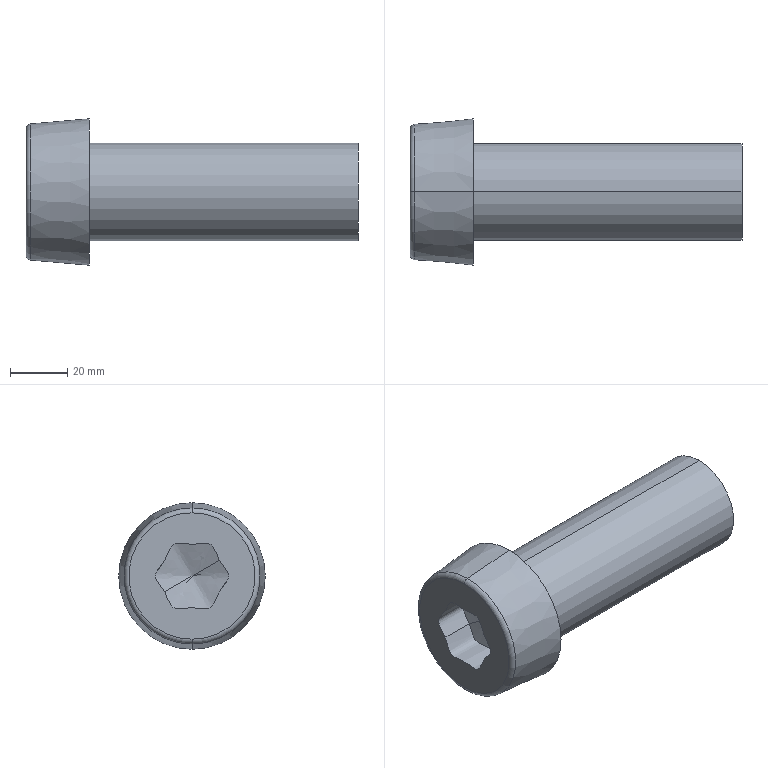Part | SolidWorks | features BlendCut 1, Cut 1, Extrusion 1, Fillet 1, LPattern 1, RevCut 1, Revolution 1, Scale 1 | 1 solid | 13 faces | box 115.6 x 51 x 51 mm | volume 120826 mm3 | spline 4 | plane 3 | torus 2 | cylinder 2 | cone 2 | commonest cylinder face diameters 34 x2
STEP:
#1=CARTESIAN_POINT('',(-21.403,-0.000002032,22.009));
#2=VERTEX_POINT('',#1);
#3=CARTESIAN_POINT('',(-21.403,-0.000002032,-22.009));
#4=VERTEX_POINT('',#3);
#5=CARTESIAN_POINT('',(-21.403,-0.000002032,0.000001814));
#6=DIRECTION('',(-1.,0.,0.));
#7=DIRECTION('',(0.,0.,-1.));
#8=AXIS2_PLACEMENT_3D('',#5,#6,#7);
#9=CIRCLE('',#8,22.009);
#10=EDGE_CURVE('',#2,#4,#9,.T.);
#11=ORIENTED_EDGE('',*,*,#10,.F.);
#12=CARTESIAN_POINT('',(-19.851,-0.000002032,23.702));
#13=VERTEX_POINT('',#12);
#14=CARTESIAN_POINT('',(-19.703,-0.000002032,22.009));
#15=DIRECTION('',(0.,1.,0.));
#16=DIRECTION('',(0.,0.,1.));
#17=AXIS2_PLACEMENT_3D('',#14,#15,#16);
#18=CIRCLE('',#17,1.7);
#19=EDGE_CURVE('',#2,#13,#18,.T.);
#20=ORIENTED_EDGE('',*,*,#19,.T.);
#21=CARTESIAN_POINT('',(-19.851,-0.000002032,-23.702));
#22=VERTEX_POINT('',#21);
#23=CARTESIAN_POINT('',(-19.851,-0.000002032,0.000001814));
#24=DIRECTION('',(1.,0.,0.));
#25=DIRECTION('',(0.,0.,-1.));
#26=AXIS2_PLACEMENT_3D('',#23,#24,#25);
#27=CIRCLE('',#26,23.702);
#28=EDGE_CURVE('',#22,#13,#27,.T.);
#29=ORIENTED_EDGE('',*,*,#28,.F.);
#30=CARTESIAN_POINT('',(-19.703,-0.000002032,-22.009));
#31=DIRECTION('',(0.,-1.,0.));
#32=DIRECTION('',(0.,0.,-1.));
#33=AXIS2_PLACEMENT_3D('',#30,#31,#32);
#34=CIRCLE('',#33,1.7);
#35=EDGE_CURVE('',#4,#22,#34,.T.);
#36=ORIENTED_EDGE('',*,*,#35,.F.);
#37=EDGE_LOOP('',(#11,#20,#29,#36));
#38=FACE_OUTER_BOUND('',#37,.T.);
#39=CARTESIAN_POINT('',(-19.703,-0.000002032,0.000001814));
#40=DIRECTION('',(1.,0.,0.));
#41=DIRECTION('',(0.,0.,-1.));
#42=AXIS2_PLACEMENT_3D('',#39,#40,#41);
#43=TOROIDAL_SURFACE('',#42,22.009,1.7);
#44=ADVANCED_FACE('',(#38),#43,.T.);
#45=CARTESIAN_POINT('',(-5.536,-0.000002032,0.000001814));
#46=VERTEX_POINT('',#45);
#47=CARTESIAN_POINT('',(-9.503,9.57,-5.525));
#48=VERTEX_POINT('',#47);
#49=CARTESIAN_POINT('',(-5.536,-0.000002032,0.000001814));
#50=CARTESIAN_POINT('',(-9.503,9.57,-5.525));
#51=B_SPLINE_CURVE_WITH_KNOTS('',1,(#49,#50),.UNSPECIFIED.,.F.,.F.,(2,2),(0.,1.),.UNSPECIFIED.);
#52=EDGE_CURVE('',#46,#48,#51,.T.);
#53=ORIENTED_EDGE('',*,*,#52,.F.);
#54=CARTESIAN_POINT('',(-9.503,-9.57,5.525));
#55=VERTEX_POINT('',#54);
#56=CARTESIAN_POINT('',(-5.536,-0.000002032,0.000001814));
#57=CARTESIAN_POINT('',(-9.503,-9.57,5.525));
#58=B_SPLINE_CURVE_WITH_KNOTS('',1,(#56,#57),.UNSPECIFIED.,.F.,.F.,(2,2),(0.,1.),.UNSPECIFIED.);
#59=EDGE_CURVE('',#46,#55,#58,.T.);
#60=ORIENTED_EDGE('',*,*,#59,.T.);
#61=CARTESIAN_POINT('',(-9.503,-9.57,5.525));
#62=CARTESIAN_POINT('',(-9.503,-8.343,7.65));
#63=CARTESIAN_POINT('',(-9.503,-7.361,12.75));
#64=CARTESIAN_POINT('',(-9.503,-0.000002032,10.2));
#65=CARTESIAN_POINT('',(-9.503,7.361,12.75));
#66=CARTESIAN_POINT('',(-9.503,8.833,5.1));
#67=CARTESIAN_POINT('',(-9.503,14.722,0.000001814));
#68=CARTESIAN_POINT('',(-9.503,10.796,-3.4));
#69=CARTESIAN_POINT('',(-9.503,9.57,-5.525));
#70=B_SPLINE_CURVE_WITH_KNOTS('',3,(#61,#62,#63,#64,#65,#66,#67,#68,#69),.UNSPECIFIED.,.F.,.F.,(4,1,1,1,1,1,4),(0.5,0.5833,0.6667,0.75,0.8333,0.9167,1.),.UNSPECIFIED.);
#71=EDGE_CURVE('',#55,#48,#70,.T.);
#72=ORIENTED_EDGE('',*,*,#71,.T.);
#73=EDGE_LOOP('',(#53,#60,#72));
#74=FACE_OUTER_BOUND('',#73,.T.);
#75=CARTESIAN_POINT('',(-5.536,-0.000002032,0.000001814));
#76=CARTESIAN_POINT('',(-9.503,9.57,-5.525));
#77=CARTESIAN_POINT('',(-5.536,-0.000002032,0.000001814));
#78=CARTESIAN_POINT('',(-9.503,8.343,-7.65));
#79=CARTESIAN_POINT('',(-5.536,-0.000002032,0.000001814));
#80=CARTESIAN_POINT('',(-9.503,7.361,-12.75));
#81=CARTESIAN_POINT('',(-5.536,-0.000002032,0.000001814));
#82=CARTESIAN_POINT('',(-9.503,-0.000002032,-10.2));
#83=CARTESIAN_POINT('',(-5.536,-0.000002032,0.000001814));
#84=CARTESIAN_POINT('',(-9.503,-7.361,-12.75));
#85=CARTESIAN_POINT('',(-5.536,-0.000002032,0.000001814));
#86=CARTESIAN_POINT('',(-9.503,-8.833,-5.1));
#87=CARTESIAN_POINT('',(-5.536,-0.000002032,0.000001814));
#88=CARTESIAN_POINT('',(-9.503,-14.722,0.000001814));
#89=CARTESIAN_POINT('',(-5.536,-0.000002032,0.000001814));
#90=CARTESIAN_POINT('',(-9.503,-8.833,5.1));
#91=CARTESIAN_POINT('',(-5.536,-0.000002032,0.000001814));
#92=CARTESIAN_POINT('',(-9.503,-7.361,12.75));
#93=CARTESIAN_POINT('',(-5.536,-0.000002032,0.000001814));
#94=CARTESIAN_POINT('',(-9.503,-0.000002032,10.2));
#95=CARTESIAN_POINT('',(-5.536,-0.000002032,0.000001814));
#96=CARTESIAN_POINT('',(-9.503,7.361,12.75));
#97=CARTESIAN_POINT('',(-5.536,-0.000002032,0.000001814));
#98=CARTESIAN_POINT('',(-9.503,8.833,5.1));
#99=CARTESIAN_POINT('',(-5.536,-0.000002032,0.000001814));
#100=CARTESIAN_POINT('',(-9.503,14.722,0.000001814));
#101=CARTESIAN_POINT('',(-5.536,-0.000002032,0.000001814));
#102=CARTESIAN_POINT('',(-9.503,10.796,-3.4));
#103=CARTESIAN_POINT('',(-5.536,-0.000002032,0.000001814));
#104=CARTESIAN_POINT('',(-9.503,9.57,-5.525));
#105=B_SPLINE_SURFACE_WITH_KNOTS('',3,1,((#75,#76),(#77,#78),(#79,#80),(#81,#82),(#83,#84),(#85,#86),(#87,#88),(#89,#90),(#91,#92),(#93,#94),(#95,#96),(#97,#98),(#99,#100),(#101,#102),(#103,#104)),.UNSPECIFIED.,.T.,.F.,.F.,(4,1,1,1,1,1,1,1,1,1,1,1,4),(2,2),(0.,0.08333,0.1667,0.25,0.3333,0.4167,0.5,0.5833,0.6667,0.75,0.8333,0.9167,1.),(0.,1.),.UNSPECIFIED.);
#106=ADVANCED_FACE('',(#74),#105,.F.);
#107=ORIENTED_EDGE('',*,*,#71,.F.);
#108=CARTESIAN_POINT('',(-21.403,-9.57,5.525));
#109=VERTEX_POINT('',#108);
#110=CARTESIAN_POINT('',(-9.503,-9.57,5.525));
#111=DIRECTION('',(-1.,0.,0.));
#112=VECTOR('',#111,1000.);
#113=LINE('',#110,#112);
#114=EDGE_CURVE('',#55,#109,#113,.T.);
#115=ORIENTED_EDGE('',*,*,#114,.T.);
#116=CARTESIAN_POINT('',(-21.403,9.57,-5.525));
#117=VERTEX_POINT('',#116);
#118=CARTESIAN_POINT('',(-21.403,9.57,-5.525));
#119=CARTESIAN_POINT('',(-21.403,10.796,-3.4));
#120=CARTESIAN_POINT('',(-21.403,14.722,0.000001814));
#121=CARTESIAN_POINT('',(-21.403,8.833,5.1));
#122=CARTESIAN_POINT('',(-21.403,7.361,12.75));
#123=CARTESIAN_POINT('',(-21.403,-0.000002032,10.2));
#124=CARTESIAN_POINT('',(-21.403,-7.361,12.75));
#125=CARTESIAN_POINT('',(-21.403,-8.343,7.65));
#126=CARTESIAN_POINT('',(-21.403,-9.57,5.525));
#127=B_SPLINE_CURVE_WITH_KNOTS('',3,(#118,#119,#120,#121,#122,#123,#124,#125,#126),.UNSPECIFIED.,.F.,.F.,(4,1,1,1,1,1,4),(0.,0.08333,0.1667,0.25,0.3333,0.4167,0.5),.UNSPECIFIED.);
#128=EDGE_CURVE('',#117,#109,#127,.T.);
#129=ORIENTED_EDGE('',*,*,#128,.F.);
#130=CARTESIAN_POINT('',(-9.503,9.57,-5.525));
#131=DIRECTION('',(-1.,0.,0.));
#132=VECTOR('',#131,1000.);
#133=LINE('',#130,#132);
#134=EDGE_CURVE('',#48,#117,#133,.T.);
#135=ORIENTED_EDGE('',*,*,#134,.F.);
#136=EDGE_LOOP('',(#107,#115,#129,#135));
#137=FACE_OUTER_BOUND('',#136,.T.);
#138=CARTESIAN_POINT('',(-9.503,9.57,-5.525));
#139=CARTESIAN_POINT('',(-21.403,9.57,-5.525));
#140=CARTESIAN_POINT('',(-9.503,10.796,-3.4));
#141=CARTESIAN_POINT('',(-21.403,10.796,-3.4));
#142=CARTESIAN_POINT('',(-9.503,14.722,0.000001814));
#143=CARTESIAN_POINT('',(-21.403,14.722,0.000001814));
#144=CARTESIAN_POINT('',(-9.503,8.833,5.1));
#145=CARTESIAN_POINT('',(-21.403,8.833,5.1));
#146=CARTESIAN_POINT('',(-9.503,7.361,12.75));
#147=CARTESIAN_POINT('',(-21.403,7.361,12.75));
#148=CARTESIAN_POINT('',(-9.503,-0.000002032,10.2));
#149=CARTESIAN_POINT('',(-21.403,-0.000002032,10.2));
#150=CARTESIAN_POINT('',(-9.503,-7.361,12.75));
#151=CARTESIAN_POINT('',(-21.403,-7.361,12.75));
#152=CARTESIAN_POINT('',(-9.503,-8.343,7.65));
#153=CARTESIAN_POINT('',(-21.403,-8.343,7.65));
#154=CARTESIAN_POINT('',(-9.503,-9.57,5.525));
#155=CARTESIAN_POINT('',(-21.403,-9.57,5.525));
#156=B_SPLINE_SURFACE_WITH_KNOTS('',3,1,((#138,#139),(#140,#141),(#142,#143),(#144,#145),(#146,#147),(#148,#149),(#150,#151),(#152,#153),(#154,#155)),.UNSPECIFIED.,.F.,.F.,.F.,(4,1,1,1,1,1,4),(2,2),(0.,0.08333,0.1667,0.25,0.3333,0.4167,0.5),(0.,1.),.UNSPECIFIED.);
#157=ADVANCED_FACE('',(#137),#156,.T.);
#158=CARTESIAN_POINT('',(94.197,-0.000002032,17.));
#159=VERTEX_POINT('',#158);
#160=CARTESIAN_POINT('',(94.197,-0.000002032,-17.));
#161=VERTEX_POINT('',#160);
#162=CARTESIAN_POINT('',(94.197,-0.000002032,0.000001814));
#163=DIRECTION('',(-1.,0.,0.));
#164=DIRECTION('',(0.,0.,1.));
#165=AXIS2_PLACEMENT_3D('',#162,#163,#164);
#166=CIRCLE('',#165,17.);
#167=EDGE_CURVE('',#159,#161,#166,.T.);
#168=ORIENTED_EDGE('',*,*,#167,.T.);
#169=CARTESIAN_POINT('',(0.6972,-0.000002032,-17.));
#170=VERTEX_POINT('',#169);
#171=CARTESIAN_POINT('',(-21.403,-0.000002032,-17.));
#172=DIRECTION('',(-1.,0.,0.));
#173=VECTOR('',#172,1000.);
#174=LINE('',#171,#173);
#175=EDGE_CURVE('',#161,#170,#174,.T.);
#176=ORIENTED_EDGE('',*,*,#175,.T.);
#177=CARTESIAN_POINT('',(0.6972,-0.000002032,17.));
#178=VERTEX_POINT('',#177);
#179=CARTESIAN_POINT('',(0.6972,-0.000002032,0.000001814));
#180=DIRECTION('',(-1.,0.,0.));
#181=DIRECTION('',(0.,0.,1.));
#182=AXIS2_PLACEMENT_3D('',#179,#180,#181);
#183=CIRCLE('',#182,17.);
#184=EDGE_CURVE('',#178,#170,#183,.T.);
#185=ORIENTED_EDGE('',*,*,#184,.F.);
#186=CARTESIAN_POINT('',(-21.403,-0.000002032,17.));
#187=DIRECTION('',(-1.,0.,0.));
#188=VECTOR('',#187,1000.);
#189=LINE('',#186,#188);
#190=EDGE_CURVE('',#159,#178,#189,.T.);
#191=ORIENTED_EDGE('',*,*,#190,.F.);
#192=EDGE_LOOP('',(#168,#176,#185,#191));
#193=FACE_OUTER_BOUND('',#192,.T.);
#194=CARTESIAN_POINT('',(-21.403,-0.000002032,0.000001814));
#195=DIRECTION('',(-1.,0.,0.));
#196=DIRECTION('',(0.,0.,1.));
#197=AXIS2_PLACEMENT_3D('',#194,#195,#196);
#198=CYLINDRICAL_SURFACE('',#197,17.);
#199=ADVANCED_FACE('',(#193),#198,.T.);
#200=ORIENTED_EDGE('',*,*,#28,.T.);
#201=CARTESIAN_POINT('',(0.6972,-0.000002032,25.5));
#202=VERTEX_POINT('',#201);
#203=CARTESIAN_POINT('',(0.6972,-0.000002032,25.5));
#204=DIRECTION('',(0.9962,0.,0.08716));
#205=VECTOR('',#204,1000.);
#206=LINE('',#203,#205);
#207=EDGE_CURVE('',#13,#202,#206,.T.);
#208=ORIENTED_EDGE('',*,*,#207,.T.);
#209=CARTESIAN_POINT('',(0.6972,-0.000002032,-25.5));
#210=VERTEX_POINT('',#209);
#211=CARTESIAN_POINT('',(0.6972,-0.000002032,0.000001814));
#212=DIRECTION('',(1.,0.,0.));
#213=DIRECTION('',(0.,0.,-1.));
#214=AXIS2_PLACEMENT_3D('',#211,#212,#213);
#215=CIRCLE('',#214,25.5);
#216=EDGE_CURVE('',#210,#202,#215,.T.);
#217=ORIENTED_EDGE('',*,*,#216,.F.);
#218=CARTESIAN_POINT('',(0.6972,-0.000002032,-25.5));
#219=DIRECTION('',(0.9962,0.,-0.08716));
#220=VECTOR('',#219,1000.);
#221=LINE('',#218,#220);
#222=EDGE_CURVE('',#22,#210,#221,.T.);
#223=ORIENTED_EDGE('',*,*,#222,.F.);
#224=EDGE_LOOP('',(#200,#208,#217,#223));
#225=FACE_OUTER_BOUND('',#224,.T.);
#226=CARTESIAN_POINT('',(0.6972,-0.000002032,0.000001814));
#227=DIRECTION('',(1.,0.,0.));
#228=DIRECTION('',(0.,0.,-1.));
#229=AXIS2_PLACEMENT_3D('',#226,#227,#228);
#230=CONICAL_SURFACE('',#229,25.5,0.08727);
#231=ADVANCED_FACE('',(#225),#230,.T.);
#232=CARTESIAN_POINT('',(-21.403,-0.000002032,0.000001814));
#233=DIRECTION('',(-1.,0.,0.));
#234=DIRECTION('',(0.,0.,-1.));
#235=AXIS2_PLACEMENT_3D('',#232,#233,#234);
#236=CIRCLE('',#235,22.009);
#237=EDGE_CURVE('',#4,#2,#236,.T.);
#238=ORIENTED_EDGE('',*,*,#237,.T.);
#239=ORIENTED_EDGE('',*,*,#10,.T.);
#240=EDGE_LOOP('',(#238,#239));
#241=FACE_OUTER_BOUND('',#240,.T.);
#242=ORIENTED_EDGE('',*,*,#128,.T.);
#243=CARTESIAN_POINT('',(-21.403,-9.57,5.525));
#244=CARTESIAN_POINT('',(-21.403,-10.796,3.4));
#245=CARTESIAN_POINT('',(-21.403,-14.722,0.000001814));
#246=CARTESIAN_POINT('',(-21.403,-8.833,-5.1));
#247=CARTESIAN_POINT('',(-21.403,-7.361,-12.75));
#248=CARTESIAN_POINT('',(-21.403,-0.000002032,-10.2));
#249=CARTESIAN_POINT('',(-21.403,7.361,-12.75));
#250=CARTESIAN_POINT('',(-21.403,8.343,-7.65));
#251=CARTESIAN_POINT('',(-21.403,9.57,-5.525));
#252=B_SPLINE_CURVE_WITH_KNOTS('',3,(#243,#244,#245,#246,#247,#248,#249,#250,#251),.UNSPECIFIED.,.F.,.F.,(4,1,1,1,1,1,4),(0.5,0.5833,0.6667,0.75,0.8333,0.9167,1.),.UNSPECIFIED.);
#253=EDGE_CURVE('',#109,#117,#252,.T.);
#254=ORIENTED_EDGE('',*,*,#253,.T.);
#255=EDGE_LOOP('',(#242,#254));
#256=FACE_BOUND('',#255,.T.);
#257=CARTESIAN_POINT('',(-21.403,-0.000002032,0.000001814));
#258=DIRECTION('',(1.,0.,0.));
#259=DIRECTION('',(0.,0.,-1.));
#260=AXIS2_PLACEMENT_3D('',#257,#258,#259);
#261=PLANE('',#260);
#262=ADVANCED_FACE('',(#241,#256),#261,.F.);
#263=ORIENTED_EDGE('',*,*,#216,.T.);
#264=CARTESIAN_POINT('',(0.6972,-0.000002032,0.000001814));
#265=DIRECTION('',(1.,0.,0.));
#266=DIRECTION('',(0.,0.,-1.));
#267=AXIS2_PLACEMENT_3D('',#264,#265,#266);
#268=CIRCLE('',#267,25.5);
#269=EDGE_CURVE('',#202,#210,#268,.T.);
#270=ORIENTED_EDGE('',*,*,#269,.T.);
#271=EDGE_LOOP('',(#263,#270));
#272=FACE_OUTER_BOUND('',#271,.T.);
#273=ORIENTED_EDGE('',*,*,#184,.T.);
#274=CARTESIAN_POINT('',(0.6972,-0.000002032,0.000001814));
#275=DIRECTION('',(-1.,0.,0.));
#276=DIRECTION('',(0.,0.,1.));
#277=AXIS2_PLACEMENT_3D('',#274,#275,#276);
#278=CIRCLE('',#277,17.);
#279=EDGE_CURVE('',#170,#178,#278,.T.);
#280=ORIENTED_EDGE('',*,*,#279,.T.);
#281=EDGE_LOOP('',(#273,#280));
#282=FACE_BOUND('',#281,.T.);
#283=CARTESIAN_POINT('',(0.6972,-0.000002032,0.000001814));
#284=DIRECTION('',(1.,0.,0.));
#285=DIRECTION('',(0.,0.,-1.));
#286=AXIS2_PLACEMENT_3D('',#283,#284,#285);
#287=PLANE('',#286);
#288=ADVANCED_FACE('',(#272,#282),#287,.T.);
#289=ORIENTED_EDGE('',*,*,#207,.F.);
#290=CARTESIAN_POINT('',(-19.851,-0.000002032,0.000001814));
#291=DIRECTION('',(1.,0.,0.));
#292=DIRECTION('',(0.,0.,-1.));
#293=AXIS2_PLACEMENT_3D('',#290,#291,#292);
#294=CIRCLE('',#293,23.702);
#295=EDGE_CURVE('',#13,#22,#294,.T.);
#296=ORIENTED_EDGE('',*,*,#295,.T.);
#297=ORIENTED_EDGE('',*,*,#222,.T.);
#298=ORIENTED_EDGE('',*,*,#269,.F.);
#299=EDGE_LOOP('',(#289,#296,#297,#298));
#300=FACE_OUTER_BOUND('',#299,.T.);
#301=CARTESIAN_POINT('',(0.6972,-0.000002032,0.000001814));
#302=DIRECTION('',(1.,0.,0.));
#303=DIRECTION('',(0.,0.,-1.));
#304=AXIS2_PLACEMENT_3D('',#301,#302,#303);
#305=CONICAL_SURFACE('',#304,25.5,0.08727);
#306=ADVANCED_FACE('',(#300),#305,.T.);
#307=ORIENTED_EDGE('',*,*,#167,.F.);
#308=CARTESIAN_POINT('',(94.197,-0.000002032,0.000001814));
#309=DIRECTION('',(-1.,0.,0.));
#310=DIRECTION('',(0.,0.,1.));
#311=AXIS2_PLACEMENT_3D('',#308,#309,#310);
#312=CIRCLE('',#311,17.);
#313=EDGE_CURVE('',#161,#159,#312,.T.);
#314=ORIENTED_EDGE('',*,*,#313,.F.);
#315=EDGE_LOOP('',(#307,#314));
#316=FACE_OUTER_BOUND('',#315,.T.);
#317=CARTESIAN_POINT('',(94.197,17.,0.000001814));
#318=DIRECTION('',(-1.,0.,0.));
#319=DIRECTION('',(0.,0.,1.));
#320=AXIS2_PLACEMENT_3D('',#317,#318,#319);
#321=PLANE('',#320);
#322=ADVANCED_FACE('',(#316),#321,.F.);
#323=ORIENTED_EDGE('',*,*,#175,.F.);
#324=ORIENTED_EDGE('',*,*,#313,.T.);
#325=ORIENTED_EDGE('',*,*,#190,.T.);
#326=ORIENTED_EDGE('',*,*,#279,.F.);
#327=EDGE_LOOP('',(#323,#324,#325,#326));
#328=FACE_OUTER_BOUND('',#327,.T.);
#329=CARTESIAN_POINT('',(-21.403,-0.000002032,0.000001814));
#330=DIRECTION('',(-1.,0.,0.));
#331=DIRECTION('',(0.,0.,1.));
#332=AXIS2_PLACEMENT_3D('',#329,#330,#331);
#333=CYLINDRICAL_SURFACE('',#332,17.);
#334=ADVANCED_FACE('',(#328),#333,.T.);
#335=ORIENTED_EDGE('',*,*,#114,.F.);
#336=CARTESIAN_POINT('',(-9.503,9.57,-5.525));
#337=CARTESIAN_POINT('',(-9.503,8.343,-7.65));
#338=CARTESIAN_POINT('',(-9.503,7.361,-12.75));
#339=CARTESIAN_POINT('',(-9.503,-0.000002032,-10.2));
#340=CARTESIAN_POINT('',(-9.503,-7.361,-12.75));
#341=CARTESIAN_POINT('',(-9.503,-8.833,-5.1));
#342=CARTESIAN_POINT('',(-9.503,-14.722,0.000001814));
#343=CARTESIAN_POINT('',(-9.503,-10.796,3.4));
#344=CARTESIAN_POINT('',(-9.503,-9.57,5.525));
#345=B_SPLINE_CURVE_WITH_KNOTS('',3,(#336,#337,#338,#339,#340,#341,#342,#343,#344),.UNSPECIFIED.,.F.,.F.,(4,1,1,1,1,1,4),(0.,0.08333,0.1667,0.25,0.3333,0.4167,0.5),.UNSPECIFIED.);
#346=EDGE_CURVE('',#48,#55,#345,.T.);
#347=ORIENTED_EDGE('',*,*,#346,.F.);
#348=ORIENTED_EDGE('',*,*,#134,.T.);
#349=ORIENTED_EDGE('',*,*,#253,.F.);
#350=EDGE_LOOP('',(#335,#347,#348,#349));
#351=FACE_OUTER_BOUND('',#350,.T.);
#352=CARTESIAN_POINT('',(-9.503,-9.57,5.525));
#353=CARTESIAN_POINT('',(-21.403,-9.57,5.525));
#354=CARTESIAN_POINT('',(-9.503,-10.796,3.4));
#355=CARTESIAN_POINT('',(-21.403,-10.796,3.4));
#356=CARTESIAN_POINT('',(-9.503,-14.722,0.000001814));
#357=CARTESIAN_POINT('',(-21.403,-14.722,0.000001814));
#358=CARTESIAN_POINT('',(-9.503,-8.833,-5.1));
#359=CARTESIAN_POINT('',(-21.403,-8.833,-5.1));
#360=CARTESIAN_POINT('',(-9.503,-7.361,-12.75));
#361=CARTESIAN_POINT('',(-21.403,-7.361,-12.75));
#362=CARTESIAN_POINT('',(-9.503,-0.000002032,-10.2));
#363=CARTESIAN_POINT('',(-21.403,-0.000002032,-10.2));
#364=CARTESIAN_POINT('',(-9.503,7.361,-12.75));
#365=CARTESIAN_POINT('',(-21.403,7.361,-12.75));
#366=CARTESIAN_POINT('',(-9.503,8.343,-7.65));
#367=CARTESIAN_POINT('',(-21.403,8.343,-7.65));
#368=CARTESIAN_POINT('',(-9.503,9.57,-5.525));
#369=CARTESIAN_POINT('',(-21.403,9.57,-5.525));
#370=B_SPLINE_SURFACE_WITH_KNOTS('',3,1,((#352,#353),(#354,#355),(#356,#357),(#358,#359),(#360,#361),(#362,#363),(#364,#365),(#366,#367),(#368,#369)),.UNSPECIFIED.,.F.,.F.,.F.,(4,1,1,1,1,1,4),(2,2),(0.5,0.5833,0.6667,0.75,0.8333,0.9167,1.),(0.,1.),.UNSPECIFIED.);
#371=ADVANCED_FACE('',(#351),#370,.T.);
#372=ORIENTED_EDGE('',*,*,#59,.F.);
#373=ORIENTED_EDGE('',*,*,#52,.T.);
#374=ORIENTED_EDGE('',*,*,#346,.T.);
#375=EDGE_LOOP('',(#372,#373,#374));
#376=FACE_OUTER_BOUND('',#375,.T.);
#377=CARTESIAN_POINT('',(-5.536,-0.000002032,0.000001814));
#378=CARTESIAN_POINT('',(-9.503,9.57,-5.525));
#379=CARTESIAN_POINT('',(-5.536,-0.000002032,0.000001814));
#380=CARTESIAN_POINT('',(-9.503,8.343,-7.65));
#381=CARTESIAN_POINT('',(-5.536,-0.000002032,0.000001814));
#382=CARTESIAN_POINT('',(-9.503,7.361,-12.75));
#383=CARTESIAN_POINT('',(-5.536,-0.000002032,0.000001814));
#384=CARTESIAN_POINT('',(-9.503,-0.000002032,-10.2));
#385=CARTESIAN_POINT('',(-5.536,-0.000002032,0.000001814));
#386=CARTESIAN_POINT('',(-9.503,-7.361,-12.75));
#387=CARTESIAN_POINT('',(-5.536,-0.000002032,0.000001814));
#388=CARTESIAN_POINT('',(-9.503,-8.833,-5.1));
#389=CARTESIAN_POINT('',(-5.536,-0.000002032,0.000001814));
#390=CARTESIAN_POINT('',(-9.503,-14.722,0.000001814));
#391=CARTESIAN_POINT('',(-5.536,-0.000002032,0.000001814));
#392=CARTESIAN_POINT('',(-9.503,-8.833,5.1));
#393=CARTESIAN_POINT('',(-5.536,-0.000002032,0.000001814));
#394=CARTESIAN_POINT('',(-9.503,-7.361,12.75));
#395=CARTESIAN_POINT('',(-5.536,-0.000002032,0.000001814));
#396=CARTESIAN_POINT('',(-9.503,-0.000002032,10.2));
#397=CARTESIAN_POINT('',(-5.536,-0.000002032,0.000001814));
#398=CARTESIAN_POINT('',(-9.503,7.361,12.75));
#399=CARTESIAN_POINT('',(-5.536,-0.000002032,0.000001814));
#400=CARTESIAN_POINT('',(-9.503,8.833,5.1));
#401=CARTESIAN_POINT('',(-5.536,-0.000002032,0.000001814));
#402=CARTESIAN_POINT('',(-9.503,14.722,0.000001814));
#403=CARTESIAN_POINT('',(-5.536,-0.000002032,0.000001814));
#404=CARTESIAN_POINT('',(-9.503,10.796,-3.4));
#405=CARTESIAN_POINT('',(-5.536,-0.000002032,0.000001814));
#406=CARTESIAN_POINT('',(-9.503,9.57,-5.525));
#407=B_SPLINE_SURFACE_WITH_KNOTS('',3,1,((#377,#378),(#379,#380),(#381,#382),(#383,#384),(#385,#386),(#387,#388),(#389,#390),(#391,#392),(#393,#394),(#395,#396),(#397,#398),(#399,#400),(#401,#402),(#403,#404),(#405,#406)),.UNSPECIFIED.,.T.,.F.,.F.,(4,1,1,1,1,1,1,1,1,1,1,1,4),(2,2),(0.,0.08333,0.1667,0.25,0.3333,0.4167,0.5,0.5833,0.6667,0.75,0.8333,0.9167,1.),(0.,1.),.UNSPECIFIED.);
#408=ADVANCED_FACE('',(#376),#407,.F.);
#409=ORIENTED_EDGE('',*,*,#19,.F.);
#410=ORIENTED_EDGE('',*,*,#237,.F.);
#411=ORIENTED_EDGE('',*,*,#35,.T.);
#412=ORIENTED_EDGE('',*,*,#295,.F.);
#413=EDGE_LOOP('',(#409,#410,#411,#412));
#414=FACE_OUTER_BOUND('',#413,.T.);
#415=CARTESIAN_POINT('',(-19.703,-0.000002032,0.000001814));
#416=DIRECTION('',(1.,0.,0.));
#417=DIRECTION('',(0.,0.,-1.));
#418=AXIS2_PLACEMENT_3D('',#415,#416,#417);
#419=TOROIDAL_SURFACE('',#418,22.009,1.7);
#420=ADVANCED_FACE('',(#414),#419,.T.);
#421=CLOSED_SHELL('',(#44,#106,#157,#199,#231,#262,#288,#306,#322,#334,#371,#408,#420));
#422=MANIFOLD_SOLID_BREP('',#421);
#423=CARTESIAN_POINT('',(0.,0.,0.));
#424=DIRECTION('',(0.,0.,1.));
#425=DIRECTION('',(1.,0.,0.));
#426=AXIS2_PLACEMENT_3D('',#423,#424,#425);
#427=(LENGTH_UNIT()NAMED_UNIT(*)SI_UNIT(.MILLI.,.METRE.));
#428=UNCERTAINTY_MEASURE_WITH_UNIT(LENGTH_MEASURE(0.00001),#427,'','');
#429=(NAMED_UNIT(*)PLANE_ANGLE_UNIT()SI_UNIT($,.RADIAN.));
#430=(NAMED_UNIT(*)SI_UNIT($,.STERADIAN.)SOLID_ANGLE_UNIT());
#431=(GEOMETRIC_REPRESENTATION_CONTEXT(3)GLOBAL_UNCERTAINTY_ASSIGNED_CONTEXT((#428))GLOBAL_UNIT_ASSIGNED_CONTEXT((#427,#429,#430))REPRESENTATION_CONTEXT('',''));
#432=ADVANCED_BREP_SHAPE_REPRESENTATION('',(#422,#426),#431);